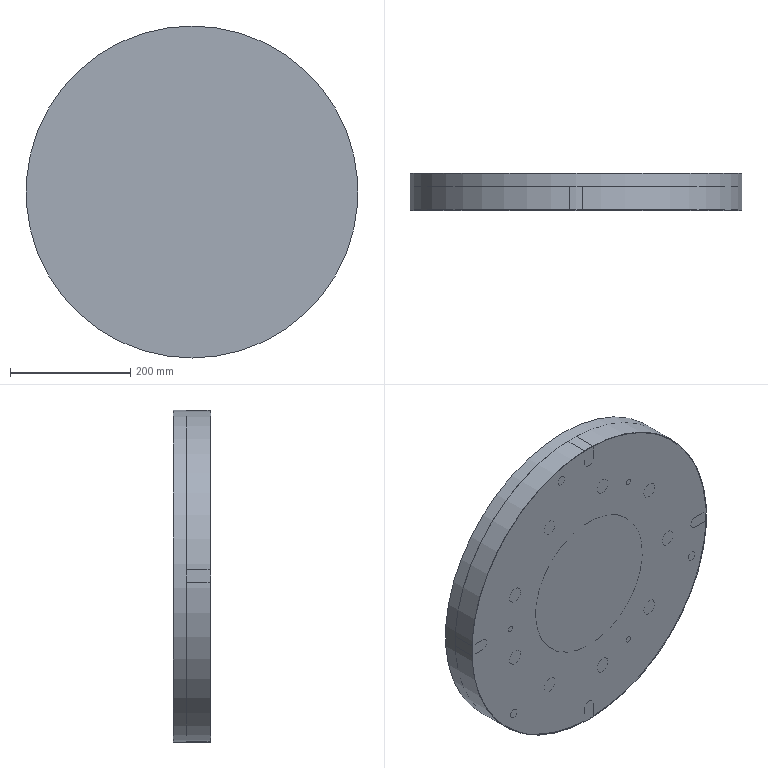NC program | NX | posted with a generic post | part box 552 x 62 x 552 mm
Whole program:
N10 G17 G21 G94 G90
(CAVITY_MILL , TOOL : D18)
N12 T02 M6
N14 G54
N16 G17 G0 G90 X0. Y-300.006 S900 M3
N18 G43 Z19. H2
N20 Z-21.5
N22 G94 G1 Z-24.5 F60.
N24 Y-249.16
N26 X-0.242 Y-249.196
N28 X-0.489 Y-249.317
N30 X-0.637 Y-249.422
N32 X-0.727 Y-249.579
N34 X-0.822 Y-249.829
N36 X-0.836 Y-249.915
N38 X-0.841 Y-250.596
N40 Y-274.783
N42 X-0.837 Y-274.846
N44 X-0.9 Y-274.843
N46 Y-270.156
N48 G3 X-5.956 Y-262.004 R9.1
N50 G2 X5.956 Y-262.004 R-13.4
N52 G3 X0.9 Y-270.156 R9.1
N54 G1 Y-274.843
N56 X0.837 Y-274.846
N58 X0.841 Y-274.783
N60 Y-250.596
N62 X0.836 Y-249.915
N64 X0.822 Y-249.829
N66 X0.727 Y-249.579
N68 X0.637 Y-249.422
N70 X0.489 Y-249.317
N72 X0.242 Y-249.196
N74 X0. Y-249.16
N76 Y-300.006
N78 Z-21.5
N80 G0 Z-24.
N82 G1 Z-27.
N84 Y-249.16
N86 X-0.242 Y-249.196
N88 X-0.489 Y-249.317
N90 X-0.637 Y-249.422
N92 X-0.727 Y-249.579
N94 X-0.822 Y-249.829
N96 X-0.836 Y-249.915
N98 X-0.841 Y-250.596
N100 Y-274.783
N102 X-0.837 Y-274.846
N104 X-0.9 Y-274.843
N106 Y-270.156
N108 G3 X-5.956 Y-262.004 R9.1
N110 G2 X5.956 Y-262.004 R-13.4
N112 G3 X0.9 Y-270.156 R9.1
N114 G1 Y-274.843
N116 X0.837 Y-274.846
N118 X0.841 Y-274.783
N120 Y-250.596
N122 X0.836 Y-249.915
N124 X0.822 Y-249.829
N126 X0.727 Y-249.579
N128 X0.637 Y-249.422
N130 X0.489 Y-249.317
N132 X0.242 Y-249.196
N134 X0. Y-249.16
N136 Y-300.006
N138 Z-24.
N140 G0 Z-26.5
N142 G1 Z-29.5
N144 Y-249.16
N146 X-0.242 Y-249.196
N148 X-0.489 Y-249.317
N150 X-0.637 Y-249.422
N152 X-0.727 Y-249.579
N154 X-0.822 Y-249.829
N156 X-0.836 Y-249.915
N158 X-0.841 Y-250.596
N160 Y-274.783
N162 X-0.837 Y-274.846
N164 X-0.9 Y-274.843
N166 Y-270.156
N168 G3 X-5.956 Y-262.004 R9.1
N170 G2 X5.956 Y-262.004 R-13.4
N172 G3 X0.9 Y-270.156 R9.1
N174 G1 Y-274.843
N176 X0.837 Y-274.846
N178 X0.841 Y-274.783
N180 Y-250.596
N182 X0.836 Y-249.915
N184 X0.822 Y-249.829
N186 X0.727 Y-249.579
N188 X0.637 Y-249.422
N190 X0.489 Y-249.317
N192 X0.242 Y-249.196
N194 X0. Y-249.16
N196 Y-300.006
N198 Z-26.5
N200 G0 Z-29.
N202 G1 Z-32.
N204 Y-249.16
N206 X-0.242 Y-249.196
N208 X-0.489 Y-249.317
N210 X-0.637 Y-249.422
N212 X-0.727 Y-249.579
N214 X-0.822 Y-249.829
N216 X-0.836 Y-249.915
N218 X-0.841 Y-250.596
N220 Y-274.783
N222 X-0.837 Y-274.846
N224 X-0.9 Y-274.843
N226 Y-270.156
N228 G3 X-5.956 Y-262.004 R9.1
N230 G2 X5.956 Y-262.004 R-13.4
N232 G3 X0.9 Y-270.156 R9.1
N234 G1 Y-274.843
N236 X0.837 Y-274.846
N238 X0.841 Y-274.783
N240 Y-250.596
N242 X0.836 Y-249.915
N244 X0.822 Y-249.829
N246 X0.727 Y-249.579
N248 X0.637 Y-249.422
N250 X0.489 Y-249.317
N252 X0.242 Y-249.196
N254 X0. Y-249.16
N256 Y-300.006
N258 Z-29.
N260 G0 Z-31.833
N262 G1 Z-34.833
N264 Y-249.16
N266 X-0.242 Y-249.196
N268 X-0.489 Y-249.317
N270 X-0.637 Y-249.422
N272 X-0.727 Y-249.579
N274 X-0.822 Y-249.829
N276 X-0.836 Y-249.915
N278 X-0.841 Y-250.596
N280 Y-274.783
N282 X-0.837 Y-274.846
N284 X-0.9 Y-274.843
N286 Y-250.
N288 G2 X0. Y-249.1 R0.9
N290 X0.9 Y-250. R0.9
N292 G1 Y-274.843
N294 X0.837 Y-274.846
N296 X0.841 Y-274.783
N298 Y-250.596
N300 X0.836 Y-249.915
N302 X0.822 Y-249.829
N304 X0.727 Y-249.579
N306 X0.637 Y-249.422
N308 X0.489 Y-249.317
N310 X0.242 Y-249.196
N312 X0. Y-249.16
N314 Y-300.006
N316 Z-31.833
N318 G0 Z-31.7
N320 Z-34.667
N322 G1 Z-37.667
N324 Y-249.16
N326 X-0.242 Y-249.196
N328 X-0.489 Y-249.317
N330 X-0.637 Y-249.422
N332 X-0.727 Y-249.579
N334 X-0.822 Y-249.829
N336 X-0.836 Y-249.915
N338 X-0.841 Y-250.596
N340 Y-274.783
N342 X-0.837 Y-274.846
N344 X-0.9 Y-274.843
N346 Y-250.
N348 G2 X0. Y-249.1 R0.9
N350 X0.9 Y-250. R0.9
N352 G1 Y-274.843
N354 X0.837 Y-274.846
N356 X0.841 Y-274.783
N358 Y-250.596
N360 X0.836 Y-249.915
N362 X0.822 Y-249.829
N364 X0.727 Y-249.579
N366 X0.637 Y-249.422
N368 X0.489 Y-249.317
N370 X0.242 Y-249.196
N372 X0. Y-249.16
N374 Y-300.006
N376 Z-34.667
N378 G0 Z-34.533
N380 Z-37.5
N382 G1 Z-40.5
N384 Y-249.16
N386 X-0.242 Y-249.196
N388 X-0.489 Y-249.317
N390 X-0.637 Y-249.422
N392 X-0.727 Y-249.579
N394 X-0.822 Y-249.829
N396 X-0.836 Y-249.915
N398 X-0.841 Y-250.596
N400 Y-274.783
N402 X-0.837 Y-274.846
N404 X-0.9 Y-274.843
N406 Y-250.
N408 G2 X0. Y-249.1 R0.9
N410 X0.9 Y-250. R0.9
N412 G1 Y-274.843
N414 X0.837 Y-274.846
N416 X0.841 Y-274.783
N418 Y-250.596
N420 X0.836 Y-249.915
N422 X0.822 Y-249.829
N424 X0.727 Y-249.579
N426 X0.637 Y-249.422
N428 X0.489 Y-249.317
N430 X0.242 Y-249.196
N432 X0. Y-249.16
N434 Y-300.006
N436 Z-37.5
N438 G0 Z-37.367
N440 Z-40.333
N442 G1 Z-43.333
N444 Y-249.16
N446 X-0.242 Y-249.196
N448 X-0.489 Y-249.317
N450 X-0.637 Y-249.422
N452 X-0.727 Y-249.579
N454 X-0.822 Y-249.829
N456 X-0.836 Y-249.915
N458 X-0.841 Y-250.596
N460 Y-274.783
N462 X-0.837 Y-274.846
N464 X-0.9 Y-274.843
N466 Y-250.
N468 G2 X0. Y-249.1 R0.9
N470 X0.9 Y-250. R0.9
N472 G1 Y-274.843
N474 X0.837 Y-274.846
N476 X0.841 Y-274.783
N478 Y-250.596
N480 X0.836 Y-249.915
N482 X0.822 Y-249.829
N484 X0.727 Y-249.579
N486 X0.637 Y-249.422
N488 X0.489 Y-249.317
N490 X0.242 Y-249.196
N492 X0. Y-249.16
N494 Y-300.006
N496 Z-40.333
N498 G0 Z-40.2
N500 Z-43.167
N502 G1 Z-46.167
N504 Y-249.16
N506 X-0.242 Y-249.196
N508 X-0.489 Y-249.317
N510 X-0.637 Y-249.422
N512 X-0.727 Y-249.579
N514 X-0.822 Y-249.829
N516 X-0.836 Y-249.915
N518 X-0.841 Y-250.596
N520 Y-274.783
N522 X-0.837 Y-274.846
N524 X-0.9 Y-274.843
N526 Y-250.
N528 G2 X0. Y-249.1 R0.9
N530 X0.9 Y-250. R0.9
N532 G1 Y-274.843
N534 X0.837 Y-274.846
N536 X0.841 Y-274.783
N538 Y-250.596
N540 X0.836 Y-249.915
N542 X0.822 Y-249.829
N544 X0.727 Y-249.579
N546 X0.637 Y-249.422
N548 X0.489 Y-249.317
N550 X0.242 Y-249.196
N552 X0. Y-249.16
N554 Y-300.006
N556 Z-43.167
N558 G0 Z-43.033
N560 Z-46.
N562 G1 Z-49.
N564 Y-249.16
N566 X-0.242 Y-249.196
N568 X-0.489 Y-249.317
N570 X-0.637 Y-249.422
N572 X-0.727 Y-249.579
N574 X-0.822 Y-249.829
N576 X-0.836 Y-249.915
N578 X-0.841 Y-250.596
N580 Y-274.783
N582 X-0.837 Y-274.846
N584 X-0.9 Y-274.843
N586 Y-250.
N588 G2 X0. Y-249.1 R0.9
N590 X0.9 Y-250. R0.9
N592 G1 Y-274.843
N594 X0.837 Y-274.846
N596 X0.841 Y-274.783
N598 Y-250.596
N600 X0.836 Y-249.915
N602 X0.822 Y-249.829
N604 X0.727 Y-249.579
N606 X0.637 Y-249.422
N608 X0.489 Y-249.317
N610 X0.242 Y-249.196
N612 X0. Y-249.16
N614 Y-300.006
N616 Z-46.
N618 G0 Z-45.867
N620 Z-48.833
N622 G1 Z-51.833
N624 Y-249.16
N626 X-0.242 Y-249.196
N628 X-0.489 Y-249.317
N630 X-0.637 Y-249.422
N632 X-0.727 Y-249.579
N634 X-0.822 Y-249.829
N636 X-0.836 Y-249.915
N638 X-0.841 Y-250.596
N640 Y-274.783
N642 X-0.837 Y-274.846
N644 X-0.9 Y-274.843
N646 Y-250.
N648 G2 X0. Y-249.1 R0.9
N650 X0.9 Y-250. R0.9
N652 G1 Y-274.843
N654 X0.837 Y-274.846
N656 X0.841 Y-274.783
N658 Y-250.596
N660 X0.836 Y-249.915
N662 X0.822 Y-249.829
N664 X0.727 Y-249.579
N666 X0.637 Y-249.422
N668 X0.489 Y-249.317
N670 X0.242 Y-249.196
N672 X0. Y-249.16
N674 Y-300.006
N676 Z-48.833
N678 G0 Z-48.7
N680 Z-51.667
N682 G1 Z-54.667
N684 Y-249.16
N686 X-0.242 Y-249.196
N688 X-0.489 Y-249.317
N690 X-0.637 Y-249.422
N692 X-0.727 Y-249.579
N694 X-0.822 Y-249.829
N696 X-0.836 Y-249.915
N698 X-0.841 Y-250.596
N700 Y-274.783
N702 X-0.837 Y-274.846
N704 X-0.9 Y-274.843
N706 Y-250.
N708 G2 X0. Y-249.1 R0.9
N710 X0.9 Y-250. R0.9
N712 G1 Y-274.843
N714 X0.837 Y-274.846
N716 X0.841 Y-274.783
N718 Y-250.596
N720 X0.836 Y-249.915
N722 X0.822 Y-249.829
N724 X0.727 Y-249.579
N726 X0.637 Y-249.422
N728 X0.489 Y-249.317
N730 X0.242 Y-249.196
N732 X0. Y-249.16
N734 Y-300.006
N736 Z-51.667
N738 G0 Z-51.533
N740 Z-54.5
N742 G1 Z-57.5
N744 Y-249.16
N746 X-0.242 Y-249.196
N748 X-0.489 Y-249.317
N750 X-0.637 Y-249.422
N752 X-0.727 Y-249.579
N754 X-0.822 Y-249.829
N756 X-0.836 Y-249.915
N758 X-0.841 Y-250.596
N760 Y-274.783
N762 X-0.837 Y-274.846
N764 X-0.9 Y-274.843
N766 Y-250.
N768 G2 X0. Y-249.1 R0.9
N770 X0.9 Y-250. R0.9
N772 G1 Y-274.843
N774 X0.837 Y-274.846
N776 X0.841 Y-274.783
N778 Y-250.596
N780 X0.836 Y-249.915
N782 X0.822 Y-249.829
N784 X0.727 Y-249.579
N786 X0.637 Y-249.422
N788 X0.489 Y-249.317
N790 X0.242 Y-249.196
N792 X0. Y-249.16
N794 Y-300.006
N796 Z-54.5
N798 G0 Z-54.367
N800 Z-57.333
N802 G1 Z-60.333
N804 Y-249.16
N806 X-0.242 Y-249.196
N808 X-0.489 Y-249.317
N810 X-0.637 Y-249.422
N812 X-0.727 Y-249.579
N814 X-0.822 Y-249.829
N816 X-0.836 Y-249.915
N818 X-0.841 Y-250.596
N820 Y-274.783
N822 X-0.837 Y-274.846
N824 X-0.9 Y-274.843
N826 Y-250.
N828 G2 X0. Y-249.1 R0.9
N830 X0.9 Y-250. R0.9
N832 G1 Y-274.843
N834 X0.837 Y-274.846
N836 X0.841 Y-274.783
N838 Y-250.596
N840 X0.836 Y-249.915
N842 X0.822 Y-249.829
N844 X0.727 Y-249.579
N846 X0.637 Y-249.422
N848 X0.489 Y-249.317
N850 X0.242 Y-249.196
N852 X0. Y-249.16
N854 Y-300.006
N856 Z-57.333
N858 G0 Z-57.2
N860 Z-60.167
N862 G1 Z-63.167
N864 Y-249.16
N866 X-0.242 Y-249.196
N868 X-0.489 Y-249.317
N870 X-0.637 Y-249.422
N872 X-0.727 Y-249.579
N874 X-0.822 Y-249.829
N876 X-0.836 Y-249.915
N878 X-0.841 Y-250.596
N880 Y-274.783
N882 X-0.837 Y-274.846
N884 X-0.9 Y-274.843
N886 Y-250.
N888 G2 X0. Y-249.1 R0.9
N890 X0.9 Y-250. R0.9
N892 G1 Y-274.843
N894 X0.837 Y-274.846
N896 X0.841 Y-274.783
N898 Y-250.596
N900 X0.836 Y-249.915
N902 X0.822 Y-249.829
N904 X0.727 Y-249.579
N906 X0.637 Y-249.422
N908 X0.489 Y-249.317
N910 X0.242 Y-249.196
N912 X0. Y-249.16
N914 Y-300.006
N916 Z-60.167
N918 G0 Z-60.033
N920 Z-63.
N922 G1 Z-66.
N924 Y-249.16
N926 X-0.242 Y-249.196
N928 X-0.489 Y-249.317
N930 X-0.637 Y-249.422
N932 X-0.727 Y-249.579
N934 X-0.822 Y-249.829
N936 X-0.836 Y-249.915
N938 X-0.841 Y-250.596
N940 Y-274.783
N942 X-0.837 Y-274.846
N944 X-0.9 Y-274.843
N946 Y-250.
N948 G2 X0. Y-249.1 R0.9
N950 X0.9 Y-250. R0.9
N952 G1 Y-274.843
N954 X0.837 Y-274.846
N956 X0.841 Y-274.783
N958 Y-250.596
N960 X0.836 Y-249.915
N962 X0.822 Y-249.829
N964 X0.727 Y-249.579
N966 X0.637 Y-249.422
N968 X0.489 Y-249.317
N970 X0.242 Y-249.196
N972 X0. Y-249.16
N974 Y-300.006
N976 Z-63.
N978 G0 Z19.
N980 M5
N982 M2